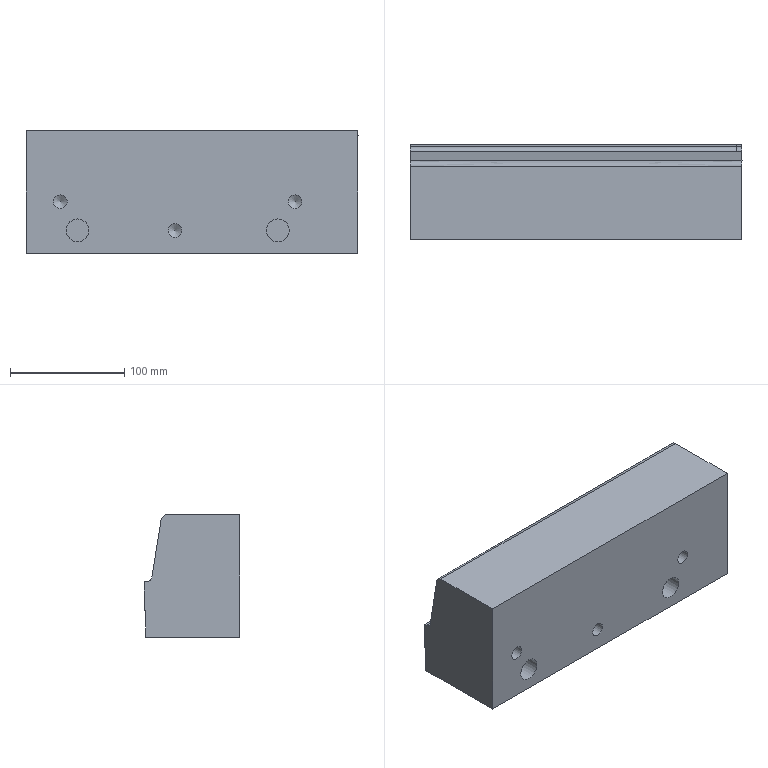Part | NX | features solid 2 | 1 solid | 24 faces | box 290 x 83.705 x 107.133 mm | volume 2376926 mm3 | plane 9 | cylinder 6 | spline 6 | cone 3 | commonest cylinder face diameters 12 x3 20 x2 10 x1
STEP:
#1=CARTESIAN_POINT('',(370.,-160.,-50.));
#2=VERTEX_POINT('',#1);
#3=CARTESIAN_POINT('',(370.,-77.709,-50.));
#4=VERTEX_POINT('',#3);
#5=CARTESIAN_POINT('',(370.,-160.,-50.));
#6=DIRECTION('',(0.,1.,0.));
#7=VECTOR('',#6,1000.);
#8=LINE('',#5,#7);
#9=EDGE_CURVE('',#2,#4,#8,.T.);
#10=ORIENTED_EDGE('',*,*,#9,.T.);
#11=CARTESIAN_POINT('',(660.,-77.708,-50.));
#12=VERTEX_POINT('',#11);
#13=CARTESIAN_POINT('',(370.,-77.709,-50.));
#14=CARTESIAN_POINT('',(466.667,-77.709,-50.));
#15=CARTESIAN_POINT('',(563.333,-77.708,-50.));
#16=CARTESIAN_POINT('',(660.,-77.708,-50.));
#17=B_SPLINE_CURVE_WITH_KNOTS('',3,(#13,#14,#15,#16),.UNSPECIFIED.,.F.,.F.,(4,4),(0.146,0.436),.UNSPECIFIED.);
#18=EDGE_CURVE('',#4,#12,#17,.T.);
#19=ORIENTED_EDGE('',*,*,#18,.T.);
#20=CARTESIAN_POINT('',(660.,-160.,-50.));
#21=VERTEX_POINT('',#20);
#22=CARTESIAN_POINT('',(660.,-75.471,-50.));
#23=DIRECTION('',(0.,1.,0.));
#24=VECTOR('',#23,1000.);
#25=LINE('',#22,#24);
#26=EDGE_CURVE('',#21,#12,#25,.T.);
#27=ORIENTED_EDGE('',*,*,#26,.F.);
#28=CARTESIAN_POINT('',(-571.479,-160.,-50.));
#29=DIRECTION('',(1.,0.,0.));
#30=VECTOR('',#29,1000.);
#31=LINE('',#28,#30);
#32=EDGE_CURVE('',#2,#21,#31,.T.);
#33=ORIENTED_EDGE('',*,*,#32,.F.);
#34=EDGE_LOOP('',(#10,#19,#27,#33));
#35=FACE_BOUND('',#34,.T.);
#36=CARTESIAN_POINT('',(-571.479,-75.471,-50.));
#37=DIRECTION('',(0.,0.,-1.));
#38=DIRECTION('',(-1.,0.,0.));
#39=AXIS2_PLACEMENT_3D('',#36,#37,#38);
#40=PLANE('',#39);
#41=ADVANCED_FACE('',(#35),#40,.T.);
#42=CARTESIAN_POINT('',(415.,-160.,-20.));
#43=VERTEX_POINT('',#42);
#44=CARTESIAN_POINT('',(415.,-160.,-30.));
#45=DIRECTION('',(0.,1.,0.));
#46=DIRECTION('',(0.,0.,1.));
#47=AXIS2_PLACEMENT_3D('',#44,#45,#46);
#48=CIRCLE('',#47,10.);
#49=EDGE_CURVE('',#43,#43,#48,.T.);
#50=ORIENTED_EDGE('',*,*,#49,.T.);
#51=EDGE_LOOP('',(#50));
#52=FACE_BOUND('',#51,.T.);
#53=CARTESIAN_POINT('',(590.,-160.,-20.));
#54=VERTEX_POINT('',#53);
#55=CARTESIAN_POINT('',(590.,-160.,-30.));
#56=DIRECTION('',(0.,1.,0.));
#57=DIRECTION('',(0.,0.,1.));
#58=AXIS2_PLACEMENT_3D('',#55,#56,#57);
#59=CIRCLE('',#58,10.);
#60=EDGE_CURVE('',#54,#54,#59,.T.);
#61=ORIENTED_EDGE('',*,*,#60,.T.);
#62=EDGE_LOOP('',(#61));
#63=FACE_BOUND('',#62,.T.);
#64=CARTESIAN_POINT('',(400.,-160.,1.));
#65=VERTEX_POINT('',#64);
#66=CARTESIAN_POINT('',(400.,-160.,-5.));
#67=DIRECTION('',(0.,1.,0.));
#68=DIRECTION('',(0.,0.,1.));
#69=AXIS2_PLACEMENT_3D('',#66,#67,#68);
#70=CIRCLE('',#69,6.);
#71=EDGE_CURVE('',#65,#65,#70,.T.);
#72=ORIENTED_EDGE('',*,*,#71,.T.);
#73=EDGE_LOOP('',(#72));
#74=FACE_BOUND('',#73,.T.);
#75=CARTESIAN_POINT('',(500.,-160.,-24.));
#76=VERTEX_POINT('',#75);
#77=CARTESIAN_POINT('',(500.,-160.,-30.));
#78=DIRECTION('',(0.,1.,0.));
#79=DIRECTION('',(0.,0.,1.));
#80=AXIS2_PLACEMENT_3D('',#77,#78,#79);
#81=CIRCLE('',#80,6.);
#82=EDGE_CURVE('',#76,#76,#81,.T.);
#83=ORIENTED_EDGE('',*,*,#82,.T.);
#84=EDGE_LOOP('',(#83));
#85=FACE_BOUND('',#84,.T.);
#86=CARTESIAN_POINT('',(605.,-160.,1.));
#87=VERTEX_POINT('',#86);
#88=CARTESIAN_POINT('',(605.,-160.,-5.));
#89=DIRECTION('',(0.,1.,0.));
#90=DIRECTION('',(0.,0.,1.));
#91=AXIS2_PLACEMENT_3D('',#88,#89,#90);
#92=CIRCLE('',#91,6.);
#93=EDGE_CURVE('',#87,#87,#92,.T.);
#94=ORIENTED_EDGE('',*,*,#93,.T.);
#95=EDGE_LOOP('',(#94));
#96=FACE_BOUND('',#95,.T.);
#97=ORIENTED_EDGE('',*,*,#32,.T.);
#98=CARTESIAN_POINT('',(660.,-160.,57.133));
#99=VERTEX_POINT('',#98);
#100=CARTESIAN_POINT('',(660.,-160.,200.));
#101=DIRECTION('',(0.,0.,-1.));
#102=VECTOR('',#101,1000.);
#103=LINE('',#100,#102);
#104=EDGE_CURVE('',#99,#21,#103,.T.);
#105=ORIENTED_EDGE('',*,*,#104,.F.);
#106=CARTESIAN_POINT('',(370.,-160.,57.133));
#107=VERTEX_POINT('',#106);
#108=CARTESIAN_POINT('',(-705.,-160.,57.133));
#109=DIRECTION('',(1.,0.,0.));
#110=VECTOR('',#109,1000.);
#111=LINE('',#108,#110);
#112=EDGE_CURVE('',#107,#99,#111,.T.);
#113=ORIENTED_EDGE('',*,*,#112,.F.);
#114=CARTESIAN_POINT('',(370.,-160.,200.));
#115=DIRECTION('',(0.,0.,1.));
#116=VECTOR('',#115,1000.);
#117=LINE('',#114,#116);
#118=EDGE_CURVE('',#2,#107,#117,.T.);
#119=ORIENTED_EDGE('',*,*,#118,.F.);
#120=EDGE_LOOP('',(#97,#105,#113,#119));
#121=FACE_BOUND('',#120,.T.);
#122=CARTESIAN_POINT('',(-705.,-160.,200.));
#123=DIRECTION('',(0.,1.,0.));
#124=DIRECTION('',(0.,0.,1.));
#125=AXIS2_PLACEMENT_3D('',#122,#123,#124);
#126=PLANE('',#125);
#127=ADVANCED_FACE('',(#52,#63,#74,#85,#96,#121),#126,.F.);
#128=CARTESIAN_POINT('',(370.,-78.294,-1.492));
#129=VERTEX_POINT('',#128);
#130=CARTESIAN_POINT('',(370.,-76.295,-1.509));
#131=VERTEX_POINT('',#130);
#132=CARTESIAN_POINT('',(370.,46.797,-2.56));
#133=DIRECTION('',(0.,1.,-0.008536));
#134=VECTOR('',#133,1000.);
#135=LINE('',#132,#134);
#136=EDGE_CURVE('',#129,#131,#135,.T.);
#137=ORIENTED_EDGE('',*,*,#136,.F.);
#138=CARTESIAN_POINT('',(655.556,-78.294,-1.492));
#139=VERTEX_POINT('',#138);
#140=CARTESIAN_POINT('',(655.556,-78.294,-1.492));
#141=CARTESIAN_POINT('',(560.371,-78.294,-1.492));
#142=CARTESIAN_POINT('',(465.185,-78.294,-1.492));
#143=CARTESIAN_POINT('',(370.,-78.294,-1.492));
#144=B_SPLINE_CURVE_WITH_KNOTS('',3,(#140,#141,#142,#143),.UNSPECIFIED.,.F.,.F.,(4,4),(0.,0.3388),.UNSPECIFIED.);
#145=EDGE_CURVE('',#139,#129,#144,.T.);
#146=ORIENTED_EDGE('',*,*,#145,.F.);
#147=CARTESIAN_POINT('',(655.585,-76.295,-1.509));
#148=VERTEX_POINT('',#147);
#149=CARTESIAN_POINT('',(655.585,-76.295,-1.509));
#150=CARTESIAN_POINT('',(655.576,-76.961,-1.503));
#151=CARTESIAN_POINT('',(655.566,-77.628,-1.498));
#152=CARTESIAN_POINT('',(655.556,-78.294,-1.492));
#153=B_SPLINE_CURVE_WITH_KNOTS('',3,(#149,#150,#151,#152),.UNSPECIFIED.,.F.,.F.,(4,4),(0.8984,1.),.UNSPECIFIED.);
#154=EDGE_CURVE('',#148,#139,#153,.T.);
#155=ORIENTED_EDGE('',*,*,#154,.F.);
#156=CARTESIAN_POINT('',(370.,-76.295,-1.509));
#157=CARTESIAN_POINT('',(465.195,-76.295,-1.509));
#158=CARTESIAN_POINT('',(560.39,-76.295,-1.509));
#159=CARTESIAN_POINT('',(655.585,-76.295,-1.509));
#160=B_SPLINE_CURVE_WITH_KNOTS('',3,(#156,#157,#158,#159),.UNSPECIFIED.,.F.,.F.,(4,4),(0.7675,1.053),.UNSPECIFIED.);
#161=EDGE_CURVE('',#131,#148,#160,.T.);
#162=ORIENTED_EDGE('',*,*,#161,.F.);
#163=EDGE_LOOP('',(#137,#146,#155,#162));
#164=FACE_BOUND('',#163,.T.);
#165=CARTESIAN_POINT('',(35.495,46.797,-2.56));
#166=DIRECTION('',(0.,-0.008536,-1.));
#167=DIRECTION('',(0.,-1.,0.008536));
#168=AXIS2_PLACEMENT_3D('',#165,#166,#167);
#169=PLANE('',#168);
#170=ADVANCED_FACE('',(#164),#169,.F.);
#171=CARTESIAN_POINT('',(370.,-83.189,2.72));
#172=VERTEX_POINT('',#171);
#173=CARTESIAN_POINT('',(370.,-78.252,3.508));
#174=DIRECTION('',(-1.,0.,0.));
#175=DIRECTION('',(0.,0.,1.));
#176=AXIS2_PLACEMENT_3D('',#173,#174,#175);
#177=CIRCLE('',#176,5.);
#178=EDGE_CURVE('',#172,#129,#177,.F.);
#179=ORIENTED_EDGE('',*,*,#178,.F.);
#180=CARTESIAN_POINT('',(655.125,-83.189,2.72));
#181=VERTEX_POINT('',#180);
#182=CARTESIAN_POINT('',(370.,-83.189,2.72));
#183=CARTESIAN_POINT('',(465.042,-83.189,2.72));
#184=CARTESIAN_POINT('',(560.083,-83.189,2.72));
#185=CARTESIAN_POINT('',(655.125,-83.189,2.72));
#186=B_SPLINE_CURVE_WITH_KNOTS('',3,(#182,#183,#184,#185),.UNSPECIFIED.,.F.,.F.,(4,4),(0.6615,1.),.UNSPECIFIED.);
#187=EDGE_CURVE('',#172,#181,#186,.T.);
#188=ORIENTED_EDGE('',*,*,#187,.T.);
#189=CARTESIAN_POINT('',(655.125,-83.189,2.72));
#190=CARTESIAN_POINT('',(655.257,-82.952,1.234));
#191=CARTESIAN_POINT('',(655.46,-81.192,-1.055));
#192=CARTESIAN_POINT('',(655.544,-79.13,-1.485));
#193=CARTESIAN_POINT('',(655.556,-78.294,-1.492));
#194=B_SPLINE_CURVE_WITH_KNOTS('',3,(#189,#190,#191,#192,#193),.UNSPECIFIED.,.F.,.F.,(4,1,4),(0.,0.5,1.),.UNSPECIFIED.);
#195=EDGE_CURVE('',#181,#139,#194,.T.);
#196=ORIENTED_EDGE('',*,*,#195,.T.);
#197=ORIENTED_EDGE('',*,*,#145,.T.);
#198=EDGE_LOOP('',(#179,#188,#196,#197));
#199=FACE_BOUND('',#198,.T.);
#200=CARTESIAN_POINT('',(6000655.556,-78.252,3.508));
#201=DIRECTION('',(-1.,0.,0.));
#202=DIRECTION('',(0.,-0.1575,0.9875));
#203=AXIS2_PLACEMENT_3D('',#200,#201,#202);
#204=CYLINDRICAL_SURFACE('',#203,5.);
#205=ADVANCED_FACE('',(#199),#204,.F.);
#206=CARTESIAN_POINT('',(370.,-91.197,52.92));
#207=VERTEX_POINT('',#206);
#208=CARTESIAN_POINT('',(660.,-91.197,52.92));
#209=VERTEX_POINT('',#208);
#210=CARTESIAN_POINT('',(370.,-91.197,52.92));
#211=CARTESIAN_POINT('',(466.667,-91.197,52.92));
#212=CARTESIAN_POINT('',(563.333,-91.197,52.92));
#213=CARTESIAN_POINT('',(660.,-91.197,52.92));
#214=B_SPLINE_CURVE_WITH_KNOTS('',3,(#210,#211,#212,#213),.UNSPECIFIED.,.F.,.F.,(4,4),(0.5681,0.8581),.UNSPECIFIED.);
#215=EDGE_CURVE('',#207,#209,#214,.T.);
#216=ORIENTED_EDGE('',*,*,#215,.F.);
#217=CARTESIAN_POINT('',(370.,-96.134,57.133));
#218=VERTEX_POINT('',#217);
#219=CARTESIAN_POINT('',(370.,-96.134,52.133));
#220=DIRECTION('',(-1.,0.,0.));
#221=DIRECTION('',(0.,0.,1.));
#222=AXIS2_PLACEMENT_3D('',#219,#220,#221);
#223=CIRCLE('',#222,5.);
#224=EDGE_CURVE('',#207,#218,#223,.F.);
#225=ORIENTED_EDGE('',*,*,#224,.T.);
#226=CARTESIAN_POINT('',(660.,-96.134,57.133));
#227=VERTEX_POINT('',#226);
#228=CARTESIAN_POINT('',(660.,-96.134,57.133));
#229=CARTESIAN_POINT('',(563.333,-96.134,57.133));
#230=CARTESIAN_POINT('',(466.667,-96.134,57.133));
#231=CARTESIAN_POINT('',(370.,-96.134,57.133));
#232=B_SPLINE_CURVE_WITH_KNOTS('',3,(#228,#229,#230,#231),.UNSPECIFIED.,.F.,.F.,(4,4),(0.08361,0.3736),.UNSPECIFIED.);
#233=EDGE_CURVE('',#227,#218,#232,.T.);
#234=ORIENTED_EDGE('',*,*,#233,.F.);
#235=CARTESIAN_POINT('',(660.,-96.134,52.133));
#236=DIRECTION('',(-1.,0.,0.));
#237=DIRECTION('',(0.,0.,1.));
#238=AXIS2_PLACEMENT_3D('',#235,#236,#237);
#239=CIRCLE('',#238,5.);
#240=EDGE_CURVE('',#227,#209,#239,.T.);
#241=ORIENTED_EDGE('',*,*,#240,.T.);
#242=EDGE_LOOP('',(#216,#225,#234,#241));
#243=FACE_BOUND('',#242,.T.);
#244=CARTESIAN_POINT('',(660.,-91.197,52.92));
#245=CARTESIAN_POINT('',(660.,-91.869,57.133));
#246=CARTESIAN_POINT('',(660.,-96.134,57.133));
#247=CARTESIAN_POINT('',(563.333,-91.197,52.92));
#248=CARTESIAN_POINT('',(563.333,-91.869,57.133));
#249=CARTESIAN_POINT('',(563.333,-96.134,57.133));
#250=CARTESIAN_POINT('',(466.667,-91.197,52.92));
#251=CARTESIAN_POINT('',(466.667,-91.869,57.133));
#252=CARTESIAN_POINT('',(466.667,-96.134,57.133));
#253=CARTESIAN_POINT('',(370.,-91.197,52.92));
#254=CARTESIAN_POINT('',(370.,-91.869,57.133));
#255=CARTESIAN_POINT('',(370.,-96.134,57.133));
#256=(BOUNDED_SURFACE()B_SPLINE_SURFACE(3,2,((#244,#245,#246),(#247,#248,#249),(#250,#251,#252),(#253,#254,#255)),.UNSPECIFIED.,.F.,.F.,.F.)B_SPLINE_SURFACE_WITH_KNOTS((4,4),(3,3),(0.1993,0.4893),(0.,1.),.PIECEWISE_BEZIER_KNOTS.)GEOMETRIC_REPRESENTATION_ITEM()RATIONAL_B_SPLINE_SURFACE(((1.,0.7608,1.),(1.,0.7608,1.),(1.,0.7608,1.),(1.,0.7608,1.)))REPRESENTATION_ITEM('')SURFACE());
#257=ADVANCED_FACE('',(#243),#256,.T.);
#258=CARTESIAN_POINT('',(370.,-87.499,29.736));
#259=DIRECTION('',(0.,0.1575,-0.9875));
#260=VECTOR('',#259,1000.);
#261=LINE('',#258,#260);
#262=EDGE_CURVE('',#207,#172,#261,.T.);
#263=ORIENTED_EDGE('',*,*,#262,.F.);
#264=ORIENTED_EDGE('',*,*,#215,.T.);
#265=CARTESIAN_POINT('',(660.,-83.189,2.72));
#266=VERTEX_POINT('',#265);
#267=CARTESIAN_POINT('',(660.,-115.038,202.387));
#268=DIRECTION('',(0.,-0.1575,0.9875));
#269=VECTOR('',#268,1000.);
#270=LINE('',#267,#269);
#271=EDGE_CURVE('',#266,#209,#270,.T.);
#272=ORIENTED_EDGE('',*,*,#271,.F.);
#273=CARTESIAN_POINT('',(655.125,-83.189,2.72));
#274=CARTESIAN_POINT('',(656.75,-83.189,2.72));
#275=CARTESIAN_POINT('',(658.375,-83.189,2.72));
#276=CARTESIAN_POINT('',(660.,-83.189,2.72));
#277=B_SPLINE_CURVE_WITH_KNOTS('',3,(#273,#274,#275,#276),.UNSPECIFIED.,.F.,.F.,(4,4),(0.9354,0.9403),.UNSPECIFIED.);
#278=EDGE_CURVE('',#181,#266,#277,.T.);
#279=ORIENTED_EDGE('',*,*,#278,.F.);
#280=ORIENTED_EDGE('',*,*,#187,.F.);
#281=EDGE_LOOP('',(#263,#264,#272,#279,#280));
#282=FACE_BOUND('',#281,.T.);
#283=CARTESIAN_POINT('',(808.196,-82.695,-0.3814));
#284=CARTESIAN_POINT('',(-199.284,-82.695,-0.3814));
#285=CARTESIAN_POINT('',(808.196,-92.303,59.853));
#286=CARTESIAN_POINT('',(-199.284,-92.303,59.853));
#287=B_SPLINE_SURFACE_WITH_KNOTS('',1,1,((#283,#284),(#285,#286)),.PLANE_SURF.,.F.,.F.,.F.,(2,2),(2,2),(-0.06964,1.283),(-0.1722,1.),.UNSPECIFIED.);
#288=ADVANCED_FACE('',(#282),#287,.F.);
#289=CARTESIAN_POINT('',(660.,-78.294,-1.492));
#290=VERTEX_POINT('',#289);
#291=CARTESIAN_POINT('',(660.,-78.252,3.508));
#292=DIRECTION('',(-1.,0.,0.));
#293=DIRECTION('',(0.,0.,1.));
#294=AXIS2_PLACEMENT_3D('',#291,#292,#293);
#295=CIRCLE('',#294,5.);
#296=EDGE_CURVE('',#290,#266,#295,.T.);
#297=ORIENTED_EDGE('',*,*,#296,.F.);
#298=CARTESIAN_POINT('',(655.556,-78.294,-1.492));
#299=CARTESIAN_POINT('',(657.037,-78.294,-1.492));
#300=CARTESIAN_POINT('',(658.519,-78.294,-1.492));
#301=CARTESIAN_POINT('',(660.,-78.294,-1.492));
#302=B_SPLINE_CURVE_WITH_KNOTS('',3,(#298,#299,#300,#301),.UNSPECIFIED.,.F.,.F.,(4,4),(0.,0.0507),.UNSPECIFIED.);
#303=EDGE_CURVE('',#139,#290,#302,.T.);
#304=ORIENTED_EDGE('',*,*,#303,.F.);
#305=ORIENTED_EDGE('',*,*,#195,.F.);
#306=ORIENTED_EDGE('',*,*,#278,.T.);
#307=EDGE_LOOP('',(#297,#304,#305,#306));
#308=FACE_BOUND('',#307,.T.);
#309=CARTESIAN_POINT('',(660.,-83.189,2.72));
#310=CARTESIAN_POINT('',(660.,-82.523,-1.456));
#311=CARTESIAN_POINT('',(660.,-78.294,-1.492));
#312=CARTESIAN_POINT('',(658.365,-83.189,2.72));
#313=CARTESIAN_POINT('',(658.365,-82.523,-1.456));
#314=CARTESIAN_POINT('',(658.365,-78.294,-1.492));
#315=CARTESIAN_POINT('',(656.73,-83.189,2.72));
#316=CARTESIAN_POINT('',(656.73,-82.523,-1.456));
#317=CARTESIAN_POINT('',(656.73,-78.294,-1.492));
#318=CARTESIAN_POINT('',(655.096,-83.189,2.72));
#319=CARTESIAN_POINT('',(655.096,-82.523,-1.456));
#320=CARTESIAN_POINT('',(655.096,-78.294,-1.492));
#321=(BOUNDED_SURFACE()B_SPLINE_SURFACE(3,2,((#309,#310,#311),(#312,#313,#314),(#315,#316,#317),(#318,#319,#320)),.UNSPECIFIED.,.F.,.F.,.F.)B_SPLINE_SURFACE_WITH_KNOTS((4,4),(3,3),(0.4131,0.418),(0.,1.),.PIECEWISE_BEZIER_KNOTS.)GEOMETRIC_REPRESENTATION_ITEM()RATIONAL_B_SPLINE_SURFACE(((1.,0.7635,1.),(1.,0.7635,1.),(1.,0.7635,1.),(1.,0.7635,1.)))REPRESENTATION_ITEM('')SURFACE());
#322=ADVANCED_FACE('',(#308),#321,.F.);
#323=CARTESIAN_POINT('',(660.,-76.295,-1.509));
#324=VERTEX_POINT('',#323);
#325=CARTESIAN_POINT('',(655.585,-76.295,-1.509));
#326=CARTESIAN_POINT('',(657.057,-76.295,-1.509));
#327=CARTESIAN_POINT('',(658.528,-76.295,-1.509));
#328=CARTESIAN_POINT('',(660.,-76.295,-1.509));
#329=B_SPLINE_CURVE_WITH_KNOTS('',3,(#325,#326,#327,#328),.UNSPECIFIED.,.F.,.F.,(4,4),(0.000855,0.00527),.UNSPECIFIED.);
#330=EDGE_CURVE('',#148,#324,#329,.T.);
#331=ORIENTED_EDGE('',*,*,#330,.F.);
#332=ORIENTED_EDGE('',*,*,#154,.T.);
#333=ORIENTED_EDGE('',*,*,#303,.T.);
#334=CARTESIAN_POINT('',(660.,-131.716,-1.036));
#335=DIRECTION('',(0.,-1.,0.008536));
#336=VECTOR('',#335,1000.);
#337=LINE('',#334,#336);
#338=EDGE_CURVE('',#324,#290,#337,.T.);
#339=ORIENTED_EDGE('',*,*,#338,.F.);
#340=EDGE_LOOP('',(#331,#332,#333,#339));
#341=FACE_BOUND('',#340,.T.);
#342=CARTESIAN_POINT('',(660.,-76.295,-1.509));
#343=CARTESIAN_POINT('',(655.53,-76.295,-1.509));
#344=CARTESIAN_POINT('',(660.,-78.294,-1.492));
#345=CARTESIAN_POINT('',(655.53,-78.294,-1.492));
#346=B_SPLINE_SURFACE_WITH_KNOTS('',1,1,((#342,#343),(#344,#345)),.PLANE_SURF.,.F.,.F.,.F.,(2,2),(2,2),(0.6913,0.7357),(0.0668,0.06988),.PIECEWISE_BEZIER_KNOTS.);
#347=ADVANCED_FACE('',(#341),#346,.F.);
#348=CARTESIAN_POINT('',(370.,-76.295,-26.51));
#349=VERTEX_POINT('',#348);
#350=CARTESIAN_POINT('',(370.,-76.295,-14.009));
#351=DIRECTION('',(0.,0.,-1.));
#352=VECTOR('',#351,1000.);
#353=LINE('',#350,#352);
#354=EDGE_CURVE('',#131,#349,#353,.T.);
#355=ORIENTED_EDGE('',*,*,#354,.F.);
#356=ORIENTED_EDGE('',*,*,#161,.T.);
#357=ORIENTED_EDGE('',*,*,#330,.T.);
#358=CARTESIAN_POINT('',(660.,-76.295,-26.51));
#359=VERTEX_POINT('',#358);
#360=CARTESIAN_POINT('',(660.,-76.295,200.));
#361=DIRECTION('',(0.,0.,-1.));
#362=VECTOR('',#361,1000.);
#363=LINE('',#360,#362);
#364=EDGE_CURVE('',#324,#359,#363,.T.);
#365=ORIENTED_EDGE('',*,*,#364,.T.);
#366=CARTESIAN_POINT('',(660.,-76.295,-26.51));
#367=CARTESIAN_POINT('',(563.333,-76.295,-26.51));
#368=CARTESIAN_POINT('',(466.667,-76.295,-26.51));
#369=CARTESIAN_POINT('',(370.,-76.295,-26.51));
#370=B_SPLINE_CURVE_WITH_KNOTS('',3,(#366,#367,#368,#369),.UNSPECIFIED.,.F.,.F.,(4,4),(0.,0.29),.UNSPECIFIED.);
#371=EDGE_CURVE('',#359,#349,#370,.T.);
#372=ORIENTED_EDGE('',*,*,#371,.T.);
#373=EDGE_LOOP('',(#355,#356,#357,#365,#372));
#374=FACE_BOUND('',#373,.T.);
#375=CARTESIAN_POINT('',(660.,-76.295,-1.509));
#376=CARTESIAN_POINT('',(660.,-76.295,-26.51));
#377=CARTESIAN_POINT('',(563.333,-76.295,-1.509));
#378=CARTESIAN_POINT('',(563.333,-76.295,-26.51));
#379=CARTESIAN_POINT('',(466.667,-76.295,-1.509));
#380=CARTESIAN_POINT('',(466.667,-76.295,-26.51));
#381=CARTESIAN_POINT('',(370.,-76.295,-1.509));
#382=CARTESIAN_POINT('',(370.,-76.295,-26.51));
#383=B_SPLINE_SURFACE_WITH_KNOTS('',3,1,((#375,#376),(#377,#378),(#379,#380),(#381,#382)),.SURF_OF_LINEAR_EXTRUSION.,.F.,.F.,.F.,(4,4),(2,2),(0.,0.2124),(0.,1.),.PIECEWISE_BEZIER_KNOTS.);
#384=ADVANCED_FACE('',(#374),#383,.F.);
#385=ORIENTED_EDGE('',*,*,#18,.F.);
#386=CARTESIAN_POINT('',(370.,-77.508,-26.5));
#387=VERTEX_POINT('',#386);
#388=CARTESIAN_POINT('',(370.,-77.709,-50.));
#389=DIRECTION('',(0.,-0.008536,-1.));
#390=VECTOR('',#389,1000.);
#391=LINE('',#388,#390);
#392=EDGE_CURVE('',#4,#387,#391,.F.);
#393=ORIENTED_EDGE('',*,*,#392,.T.);
#394=CARTESIAN_POINT('',(660.,-77.508,-26.5));
#395=VERTEX_POINT('',#394);
#396=CARTESIAN_POINT('',(660.,-77.508,-26.5));
#397=CARTESIAN_POINT('',(563.333,-77.508,-26.5));
#398=CARTESIAN_POINT('',(466.667,-77.508,-26.5));
#399=CARTESIAN_POINT('',(370.,-77.508,-26.5));
#400=B_SPLINE_CURVE_WITH_KNOTS('',3,(#396,#397,#398,#399),.UNSPECIFIED.,.F.,.F.,(4,4),(1.305,1.595),.UNSPECIFIED.);
#401=EDGE_CURVE('',#387,#395,#400,.F.);
#402=ORIENTED_EDGE('',*,*,#401,.T.);
#403=CARTESIAN_POINT('',(660.,-77.608,-38.267));
#404=DIRECTION('',(0.,-0.008536,-1.));
#405=VECTOR('',#404,1000.);
#406=LINE('',#403,#405);
#407=EDGE_CURVE('',#395,#12,#406,.T.);
#408=ORIENTED_EDGE('',*,*,#407,.T.);
#409=EDGE_LOOP('',(#385,#393,#402,#408));
#410=FACE_BOUND('',#409,.T.);
#411=CARTESIAN_POINT('',(370.,-77.508,-26.5));
#412=CARTESIAN_POINT('',(370.,-77.709,-50.));
#413=CARTESIAN_POINT('',(466.667,-77.508,-26.5));
#414=CARTESIAN_POINT('',(466.667,-77.709,-50.));
#415=CARTESIAN_POINT('',(563.333,-77.508,-26.5));
#416=CARTESIAN_POINT('',(563.333,-77.708,-50.));
#417=CARTESIAN_POINT('',(660.,-77.508,-26.5));
#418=CARTESIAN_POINT('',(660.,-77.708,-50.));
#419=B_SPLINE_SURFACE_WITH_KNOTS('',3,1,((#411,#412),(#413,#414),(#415,#416),(#417,#418)),.SURF_OF_LINEAR_EXTRUSION.,.F.,.F.,.F.,(4,4),(2,2),(0.7876,1.),(0.,1.),.PIECEWISE_BEZIER_KNOTS.);
#420=ADVANCED_FACE('',(#410),#419,.T.);
#421=ORIENTED_EDGE('',*,*,#401,.F.);
#422=CARTESIAN_POINT('',(370.,-76.914,-26.505));
#423=DIRECTION('',(0.,-1.,0.008536));
#424=VECTOR('',#423,1000.);
#425=LINE('',#422,#424);
#426=EDGE_CURVE('',#349,#387,#425,.T.);
#427=ORIENTED_EDGE('',*,*,#426,.F.);
#428=ORIENTED_EDGE('',*,*,#371,.F.);
#429=CARTESIAN_POINT('',(660.,-131.93,-26.035));
#430=DIRECTION('',(0.,1.,-0.008536));
#431=VECTOR('',#430,1000.);
#432=LINE('',#429,#431);
#433=EDGE_CURVE('',#395,#359,#432,.T.);
#434=ORIENTED_EDGE('',*,*,#433,.F.);
#435=EDGE_LOOP('',(#421,#427,#428,#434));
#436=FACE_BOUND('',#435,.T.);
#437=CARTESIAN_POINT('',(-437.652,-76.914,-26.505));
#438=DIRECTION('',(0.,0.008536,1.));
#439=DIRECTION('',(0.,-1.,0.008536));
#440=AXIS2_PLACEMENT_3D('',#437,#438,#439);
#441=PLANE('',#440);
#442=ADVANCED_FACE('',(#436),#441,.F.);
#443=ORIENTED_EDGE('',*,*,#426,.T.);
#444=ORIENTED_EDGE('',*,*,#392,.F.);
#445=ORIENTED_EDGE('',*,*,#9,.F.);
#446=ORIENTED_EDGE('',*,*,#118,.T.);
#447=CARTESIAN_POINT('',(370.,-91.869,57.133));
#448=DIRECTION('',(0.,-1.,0.));
#449=VECTOR('',#448,1000.);
#450=LINE('',#447,#449);
#451=EDGE_CURVE('',#218,#107,#450,.T.);
#452=ORIENTED_EDGE('',*,*,#451,.F.);
#453=ORIENTED_EDGE('',*,*,#224,.F.);
#454=ORIENTED_EDGE('',*,*,#262,.T.);
#455=ORIENTED_EDGE('',*,*,#178,.T.);
#456=ORIENTED_EDGE('',*,*,#136,.T.);
#457=ORIENTED_EDGE('',*,*,#354,.T.);
#458=EDGE_LOOP('',(#443,#444,#445,#446,#452,#453,#454,#455,#456,#457));
#459=FACE_BOUND('',#458,.T.);
#460=CARTESIAN_POINT('',(370.,360.,0.));
#461=DIRECTION('',(-1.,0.,0.));
#462=DIRECTION('',(0.,0.,1.));
#463=AXIS2_PLACEMENT_3D('',#460,#461,#462);
#464=PLANE('',#463);
#465=ADVANCED_FACE('',(#459),#464,.T.);
#466=ORIENTED_EDGE('',*,*,#233,.T.);
#467=ORIENTED_EDGE('',*,*,#451,.T.);
#468=ORIENTED_EDGE('',*,*,#112,.T.);
#469=CARTESIAN_POINT('',(660.,-130.,57.133));
#470=DIRECTION('',(0.,1.,0.));
#471=VECTOR('',#470,1000.);
#472=LINE('',#469,#471);
#473=EDGE_CURVE('',#99,#227,#472,.T.);
#474=ORIENTED_EDGE('',*,*,#473,.T.);
#475=EDGE_LOOP('',(#466,#467,#468,#474));
#476=FACE_BOUND('',#475,.T.);
#477=CARTESIAN_POINT('',(743.607,-91.869,57.133));
#478=DIRECTION('',(0.,0.,1.));
#479=DIRECTION('',(1.,0.,0.));
#480=AXIS2_PLACEMENT_3D('',#477,#478,#479);
#481=PLANE('',#480);
#482=ADVANCED_FACE('',(#476),#481,.T.);
#483=ORIENTED_EDGE('',*,*,#104,.T.);
#484=ORIENTED_EDGE('',*,*,#26,.T.);
#485=ORIENTED_EDGE('',*,*,#407,.F.);
#486=ORIENTED_EDGE('',*,*,#433,.T.);
#487=ORIENTED_EDGE('',*,*,#364,.F.);
#488=ORIENTED_EDGE('',*,*,#338,.T.);
#489=ORIENTED_EDGE('',*,*,#296,.T.);
#490=ORIENTED_EDGE('',*,*,#271,.T.);
#491=ORIENTED_EDGE('',*,*,#240,.F.);
#492=ORIENTED_EDGE('',*,*,#473,.F.);
#493=EDGE_LOOP('',(#483,#484,#485,#486,#487,#488,#489,#490,#491,#492));
#494=FACE_BOUND('',#493,.T.);
#495=CARTESIAN_POINT('',(660.,-130.,200.));
#496=DIRECTION('',(-1.,0.,0.));
#497=DIRECTION('',(0.,0.,1.));
#498=AXIS2_PLACEMENT_3D('',#495,#496,#497);
#499=PLANE('',#498);
#500=ADVANCED_FACE('',(#494),#499,.F.);
#501=CARTESIAN_POINT('',(605.,-130.,1.));
#502=VERTEX_POINT('',#501);
#503=CARTESIAN_POINT('',(605.,-130.,-5.));
#504=DIRECTION('',(0.,1.,0.));
#505=DIRECTION('',(0.,0.,1.));
#506=AXIS2_PLACEMENT_3D('',#503,#504,#505);
#507=CIRCLE('',#506,6.);
#508=EDGE_CURVE('',#502,#502,#507,.T.);
#509=ORIENTED_EDGE('',*,*,#508,.F.);
#510=EDGE_LOOP('',(#509));
#511=FACE_BOUND('',#510,.T.);
#512=CARTESIAN_POINT('',(605.,-126.395,-5.));
#513=VERTEX_POINT('',#512);
#514=VERTEX_LOOP('',#513);
#515=FACE_BOUND('',#514,.T.);
#516=CARTESIAN_POINT('',(605.,-130.,-5.));
#517=DIRECTION('',(0.,-1.,0.));
#518=DIRECTION('',(0.,0.,-1.));
#519=AXIS2_PLACEMENT_3D('',#516,#517,#518);
#520=CONICAL_SURFACE('',#519,6.,1.03);
#521=ADVANCED_FACE('',(#511,#515),#520,.F.);
#522=ORIENTED_EDGE('',*,*,#508,.T.);
#523=EDGE_LOOP('',(#522));
#524=FACE_BOUND('',#523,.T.);
#525=ORIENTED_EDGE('',*,*,#93,.F.);
#526=EDGE_LOOP('',(#525));
#527=FACE_BOUND('',#526,.T.);
#528=CARTESIAN_POINT('',(605.,-160.,-5.));
#529=DIRECTION('',(0.,1.,0.));
#530=DIRECTION('',(0.,0.,1.));
#531=AXIS2_PLACEMENT_3D('',#528,#529,#530);
#532=CYLINDRICAL_SURFACE('',#531,6.);
#533=ADVANCED_FACE('',(#524,#527),#532,.F.);
#534=CARTESIAN_POINT('',(500.,-130.,-24.));
#535=VERTEX_POINT('',#534);
#536=CARTESIAN_POINT('',(500.,-130.,-30.));
#537=DIRECTION('',(0.,1.,0.));
#538=DIRECTION('',(0.,0.,1.));
#539=AXIS2_PLACEMENT_3D('',#536,#537,#538);
#540=CIRCLE('',#539,6.);
#541=EDGE_CURVE('',#535,#535,#540,.T.);
#542=ORIENTED_EDGE('',*,*,#541,.F.);
#543=EDGE_LOOP('',(#542));
#544=FACE_BOUND('',#543,.T.);
#545=CARTESIAN_POINT('',(500.,-126.395,-30.));
#546=VERTEX_POINT('',#545);
#547=VERTEX_LOOP('',#546);
#548=FACE_BOUND('',#547,.T.);
#549=CARTESIAN_POINT('',(500.,-130.,-30.));
#550=DIRECTION('',(0.,-1.,0.));
#551=DIRECTION('',(0.,0.,-1.));
#552=AXIS2_PLACEMENT_3D('',#549,#550,#551);
#553=CONICAL_SURFACE('',#552,6.,1.03);
#554=ADVANCED_FACE('',(#544,#548),#553,.F.);
#555=ORIENTED_EDGE('',*,*,#541,.T.);
#556=EDGE_LOOP('',(#555));
#557=FACE_BOUND('',#556,.T.);
#558=ORIENTED_EDGE('',*,*,#82,.F.);
#559=EDGE_LOOP('',(#558));
#560=FACE_BOUND('',#559,.T.);
#561=CARTESIAN_POINT('',(500.,-160.,-30.));
#562=DIRECTION('',(0.,1.,0.));
#563=DIRECTION('',(0.,0.,1.));
#564=AXIS2_PLACEMENT_3D('',#561,#562,#563);
#565=CYLINDRICAL_SURFACE('',#564,6.);
#566=ADVANCED_FACE('',(#557,#560),#565,.F.);
#567=CARTESIAN_POINT('',(400.,-130.,1.));
#568=VERTEX_POINT('',#567);
#569=CARTESIAN_POINT('',(400.,-130.,-5.));
#570=DIRECTION('',(0.,1.,0.));
#571=DIRECTION('',(0.,0.,1.));
#572=AXIS2_PLACEMENT_3D('',#569,#570,#571);
#573=CIRCLE('',#572,6.);
#574=EDGE_CURVE('',#568,#568,#573,.T.);
#575=ORIENTED_EDGE('',*,*,#574,.F.);
#576=EDGE_LOOP('',(#575));
#577=FACE_BOUND('',#576,.T.);
#578=CARTESIAN_POINT('',(400.,-126.395,-5.));
#579=VERTEX_POINT('',#578);
#580=VERTEX_LOOP('',#579);
#581=FACE_BOUND('',#580,.T.);
#582=CARTESIAN_POINT('',(400.,-130.,-5.));
#583=DIRECTION('',(0.,-1.,0.));
#584=DIRECTION('',(0.,0.,-1.));
#585=AXIS2_PLACEMENT_3D('',#582,#583,#584);
#586=CONICAL_SURFACE('',#585,6.,1.03);
#587=ADVANCED_FACE('',(#577,#581),#586,.F.);
#588=ORIENTED_EDGE('',*,*,#574,.T.);
#589=EDGE_LOOP('',(#588));
#590=FACE_BOUND('',#589,.T.);
#591=ORIENTED_EDGE('',*,*,#71,.F.);
#592=EDGE_LOOP('',(#591));
#593=FACE_BOUND('',#592,.T.);
#594=CARTESIAN_POINT('',(400.,-160.,-5.));
#595=DIRECTION('',(0.,1.,0.));
#596=DIRECTION('',(0.,0.,1.));
#597=AXIS2_PLACEMENT_3D('',#594,#595,#596);
#598=CYLINDRICAL_SURFACE('',#597,6.);
#599=ADVANCED_FACE('',(#590,#593),#598,.F.);
#600=CARTESIAN_POINT('',(590.,-130.,-20.));
#601=VERTEX_POINT('',#600);
#602=CARTESIAN_POINT('',(590.,-130.,-30.));
#603=DIRECTION('',(0.,1.,0.));
#604=DIRECTION('',(0.,0.,1.));
#605=AXIS2_PLACEMENT_3D('',#602,#603,#604);
#606=CIRCLE('',#605,10.);
#607=EDGE_CURVE('',#601,#601,#606,.T.);
#608=ORIENTED_EDGE('',*,*,#607,.T.);
#609=EDGE_LOOP('',(#608));
#610=FACE_BOUND('',#609,.T.);
#611=ORIENTED_EDGE('',*,*,#60,.F.);
#612=EDGE_LOOP('',(#611));
#613=FACE_BOUND('',#612,.T.);
#614=CARTESIAN_POINT('',(590.,-160.,-30.));
#615=DIRECTION('',(0.,1.,0.));
#616=DIRECTION('',(0.,0.,1.));
#617=AXIS2_PLACEMENT_3D('',#614,#615,#616);
#618=CYLINDRICAL_SURFACE('',#617,10.);
#619=ADVANCED_FACE('',(#610,#613),#618,.F.);
#620=ORIENTED_EDGE('',*,*,#607,.F.);
#621=EDGE_LOOP('',(#620));
#622=FACE_BOUND('',#621,.T.);
#623=CARTESIAN_POINT('',(590.,-130.,-30.));
#624=DIRECTION('',(0.,1.,0.));
#625=DIRECTION('',(0.,0.,1.));
#626=AXIS2_PLACEMENT_3D('',#623,#624,#625);
#627=PLANE('',#626);
#628=ADVANCED_FACE('',(#622),#627,.F.);
#629=CARTESIAN_POINT('',(415.,-130.,-20.));
#630=VERTEX_POINT('',#629);
#631=CARTESIAN_POINT('',(415.,-130.,-30.));
#632=DIRECTION('',(0.,1.,0.));
#633=DIRECTION('',(0.,0.,1.));
#634=AXIS2_PLACEMENT_3D('',#631,#632,#633);
#635=CIRCLE('',#634,10.);
#636=EDGE_CURVE('',#630,#630,#635,.T.);
#637=ORIENTED_EDGE('',*,*,#636,.T.);
#638=EDGE_LOOP('',(#637));
#639=FACE_BOUND('',#638,.T.);
#640=ORIENTED_EDGE('',*,*,#49,.F.);
#641=EDGE_LOOP('',(#640));
#642=FACE_BOUND('',#641,.T.);
#643=CARTESIAN_POINT('',(415.,-160.,-30.));
#644=DIRECTION('',(0.,1.,0.));
#645=DIRECTION('',(0.,0.,1.));
#646=AXIS2_PLACEMENT_3D('',#643,#644,#645);
#647=CYLINDRICAL_SURFACE('',#646,10.);
#648=ADVANCED_FACE('',(#639,#642),#647,.F.);
#649=ORIENTED_EDGE('',*,*,#636,.F.);
#650=EDGE_LOOP('',(#649));
#651=FACE_BOUND('',#650,.T.);
#652=CARTESIAN_POINT('',(415.,-130.,-30.));
#653=DIRECTION('',(0.,1.,0.));
#654=DIRECTION('',(0.,0.,1.));
#655=AXIS2_PLACEMENT_3D('',#652,#653,#654);
#656=PLANE('',#655);
#657=ADVANCED_FACE('',(#651),#656,.F.);
#658=CLOSED_SHELL('',(#41,#127,#170,#205,#257,#288,#322,#347,#384,#420,#442,#465,#482,#500,#521,#533,#554,#566,#587,#599,#619,#628,#648,#657));
#659=MANIFOLD_SOLID_BREP('',#658);
#660=(LENGTH_UNIT()NAMED_UNIT(*)SI_UNIT(.MILLI.,.METRE.));
#661=UNCERTAINTY_MEASURE_WITH_UNIT(LENGTH_MEASURE(0.0508),#660,'','');
#662=(NAMED_UNIT(*)PLANE_ANGLE_UNIT()SI_UNIT($,.RADIAN.));
#663=(NAMED_UNIT(*)SI_UNIT($,.STERADIAN.)SOLID_ANGLE_UNIT());
#664=(GEOMETRIC_REPRESENTATION_CONTEXT(3)GLOBAL_UNCERTAINTY_ASSIGNED_CONTEXT((#661))GLOBAL_UNIT_ASSIGNED_CONTEXT((#660,#662,#663))REPRESENTATION_CONTEXT('',''));
#665=ADVANCED_BREP_SHAPE_REPRESENTATION('',(#659),#664);